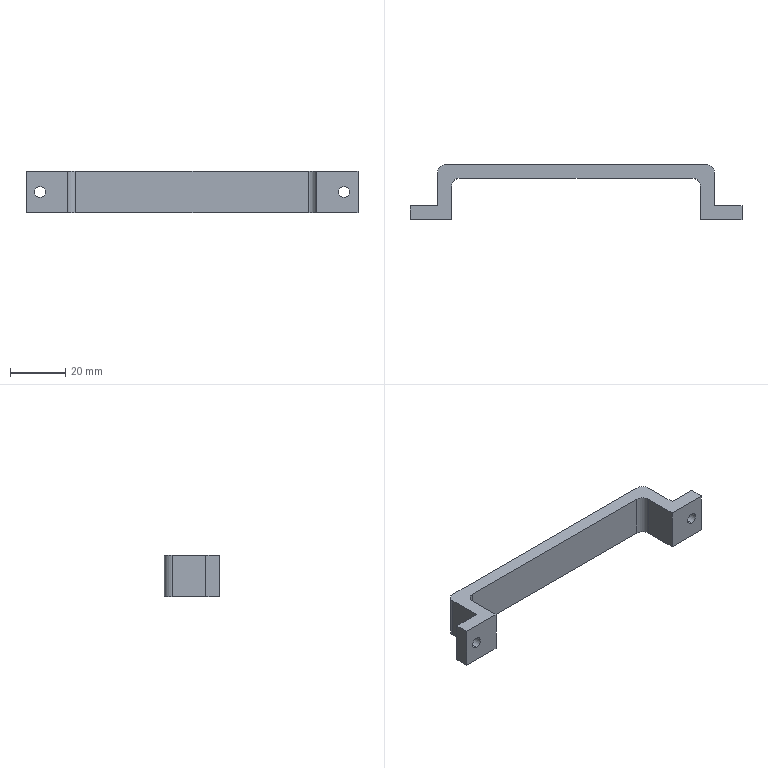Part | SolidWorks | features Extrusion 1, Fillet 1, ICE 1 | 1 solid | 22 faces | box 120 x 20 x 15 mm | volume 11124 mm3 | plane 14 | cylinder 8 | commonest cylinder face diameters 4 x4 6 x4
STEP:
#1=CARTESIAN_POINT('',(115.,0.,5.5));
#2=VERTEX_POINT('',#1);
#3=CARTESIAN_POINT('',(115.,0.,9.5));
#4=VERTEX_POINT('',#3);
#5=CARTESIAN_POINT('',(115.,0.,7.5));
#6=DIRECTION('',(0.,1.,0.));
#7=DIRECTION('',(0.,0.,1.));
#8=AXIS2_PLACEMENT_3D('',#5,#6,#7);
#9=CIRCLE('',#8,2.);
#10=EDGE_CURVE('',#2,#4,#9,.T.);
#11=ORIENTED_EDGE('',*,*,#10,.F.);
#12=CARTESIAN_POINT('',(115.,5.,5.5));
#13=VERTEX_POINT('',#12);
#14=CARTESIAN_POINT('',(115.,-10.,5.5));
#15=DIRECTION('',(0.,1.,0.));
#16=VECTOR('',#15,1000.);
#17=LINE('',#14,#16);
#18=EDGE_CURVE('',#2,#13,#17,.T.);
#19=ORIENTED_EDGE('',*,*,#18,.T.);
#20=CARTESIAN_POINT('',(115.,5.,9.5));
#21=VERTEX_POINT('',#20);
#22=CARTESIAN_POINT('',(115.,5.,7.5));
#23=DIRECTION('',(0.,1.,0.));
#24=DIRECTION('',(0.,0.,1.));
#25=AXIS2_PLACEMENT_3D('',#22,#23,#24);
#26=CIRCLE('',#25,2.);
#27=EDGE_CURVE('',#13,#21,#26,.T.);
#28=ORIENTED_EDGE('',*,*,#27,.T.);
#29=CARTESIAN_POINT('',(115.,-10.,9.5));
#30=DIRECTION('',(0.,1.,0.));
#31=VECTOR('',#30,1000.);
#32=LINE('',#29,#31);
#33=EDGE_CURVE('',#4,#21,#32,.T.);
#34=ORIENTED_EDGE('',*,*,#33,.F.);
#35=EDGE_LOOP('',(#11,#19,#28,#34));
#36=FACE_OUTER_BOUND('',#35,.T.);
#37=CARTESIAN_POINT('',(115.,-10.,7.5));
#38=DIRECTION('',(0.,1.,0.));
#39=DIRECTION('',(0.,0.,1.));
#40=AXIS2_PLACEMENT_3D('',#37,#38,#39);
#41=CYLINDRICAL_SURFACE('',#40,2.);
#42=ADVANCED_FACE('',(#36),#41,.F.);
#43=CARTESIAN_POINT('',(5.,0.,5.5));
#44=VERTEX_POINT('',#43);
#45=CARTESIAN_POINT('',(5.,0.,9.5));
#46=VERTEX_POINT('',#45);
#47=CARTESIAN_POINT('',(5.,0.,7.5));
#48=DIRECTION('',(0.,1.,0.));
#49=DIRECTION('',(0.,0.,1.));
#50=AXIS2_PLACEMENT_3D('',#47,#48,#49);
#51=CIRCLE('',#50,2.);
#52=EDGE_CURVE('',#44,#46,#51,.T.);
#53=ORIENTED_EDGE('',*,*,#52,.F.);
#54=CARTESIAN_POINT('',(5.,5.,5.5));
#55=VERTEX_POINT('',#54);
#56=CARTESIAN_POINT('',(5.,-10.,5.5));
#57=DIRECTION('',(0.,1.,0.));
#58=VECTOR('',#57,1000.);
#59=LINE('',#56,#58);
#60=EDGE_CURVE('',#44,#55,#59,.T.);
#61=ORIENTED_EDGE('',*,*,#60,.T.);
#62=CARTESIAN_POINT('',(5.,5.,9.5));
#63=VERTEX_POINT('',#62);
#64=CARTESIAN_POINT('',(5.,5.,7.5));
#65=DIRECTION('',(0.,1.,0.));
#66=DIRECTION('',(0.,0.,1.));
#67=AXIS2_PLACEMENT_3D('',#64,#65,#66);
#68=CIRCLE('',#67,2.);
#69=EDGE_CURVE('',#55,#63,#68,.T.);
#70=ORIENTED_EDGE('',*,*,#69,.T.);
#71=CARTESIAN_POINT('',(5.,-10.,9.5));
#72=DIRECTION('',(0.,1.,0.));
#73=VECTOR('',#72,1000.);
#74=LINE('',#71,#73);
#75=EDGE_CURVE('',#46,#63,#74,.T.);
#76=ORIENTED_EDGE('',*,*,#75,.F.);
#77=EDGE_LOOP('',(#53,#61,#70,#76));
#78=FACE_OUTER_BOUND('',#77,.T.);
#79=CARTESIAN_POINT('',(5.,-10.,7.5));
#80=DIRECTION('',(0.,1.,0.));
#81=DIRECTION('',(0.,0.,1.));
#82=AXIS2_PLACEMENT_3D('',#79,#80,#81);
#83=CYLINDRICAL_SURFACE('',#82,2.);
#84=ADVANCED_FACE('',(#78),#83,.F.);
#85=CARTESIAN_POINT('',(0.,5.,0.));
#86=VERTEX_POINT('',#85);
#87=CARTESIAN_POINT('',(0.,0.,0.));
#88=VERTEX_POINT('',#87);
#89=CARTESIAN_POINT('',(0.,0.,0.));
#90=DIRECTION('',(0.,-1.,0.));
#91=VECTOR('',#90,1000.);
#92=LINE('',#89,#91);
#93=EDGE_CURVE('',#86,#88,#92,.T.);
#94=ORIENTED_EDGE('',*,*,#93,.T.);
#95=CARTESIAN_POINT('',(0.,0.,15.));
#96=VERTEX_POINT('',#95);
#97=CARTESIAN_POINT('',(0.,0.,15.));
#98=DIRECTION('',(0.,0.,-1.));
#99=VECTOR('',#98,1000.);
#100=LINE('',#97,#99);
#101=EDGE_CURVE('',#96,#88,#100,.T.);
#102=ORIENTED_EDGE('',*,*,#101,.F.);
#103=CARTESIAN_POINT('',(0.,5.,15.));
#104=VERTEX_POINT('',#103);
#105=CARTESIAN_POINT('',(0.,0.,15.));
#106=DIRECTION('',(0.,-1.,0.));
#107=VECTOR('',#106,1000.);
#108=LINE('',#105,#107);
#109=EDGE_CURVE('',#104,#96,#108,.T.);
#110=ORIENTED_EDGE('',*,*,#109,.F.);
#111=CARTESIAN_POINT('',(0.,5.,15.));
#112=DIRECTION('',(0.,0.,-1.));
#113=VECTOR('',#112,1000.);
#114=LINE('',#111,#113);
#115=EDGE_CURVE('',#104,#86,#114,.T.);
#116=ORIENTED_EDGE('',*,*,#115,.T.);
#117=EDGE_LOOP('',(#94,#102,#110,#116));
#118=FACE_OUTER_BOUND('',#117,.T.);
#119=CARTESIAN_POINT('',(0.,0.,15.));
#120=DIRECTION('',(1.,0.,0.));
#121=DIRECTION('',(0.,0.,-1.));
#122=AXIS2_PLACEMENT_3D('',#119,#120,#121);
#123=PLANE('',#122);
#124=ADVANCED_FACE('',(#118),#123,.F.);
#125=CARTESIAN_POINT('',(5.,0.,7.5));
#126=DIRECTION('',(0.,1.,0.));
#127=DIRECTION('',(0.,0.,1.));
#128=AXIS2_PLACEMENT_3D('',#125,#126,#127);
#129=CIRCLE('',#128,2.);
#130=EDGE_CURVE('',#46,#44,#129,.T.);
#131=ORIENTED_EDGE('',*,*,#130,.T.);
#132=ORIENTED_EDGE('',*,*,#52,.T.);
#133=EDGE_LOOP('',(#131,#132));
#134=FACE_BOUND('',#133,.T.);
#135=CARTESIAN_POINT('',(15.,0.,0.));
#136=VERTEX_POINT('',#135);
#137=CARTESIAN_POINT('',(0.,0.,0.));
#138=DIRECTION('',(1.,0.,0.));
#139=VECTOR('',#138,1000.);
#140=LINE('',#137,#139);
#141=EDGE_CURVE('',#88,#136,#140,.T.);
#142=ORIENTED_EDGE('',*,*,#141,.T.);
#143=CARTESIAN_POINT('',(15.,0.,15.));
#144=VERTEX_POINT('',#143);
#145=CARTESIAN_POINT('',(15.,0.,15.));
#146=DIRECTION('',(0.,0.,-1.));
#147=VECTOR('',#146,1000.);
#148=LINE('',#145,#147);
#149=EDGE_CURVE('',#144,#136,#148,.T.);
#150=ORIENTED_EDGE('',*,*,#149,.F.);
#151=CARTESIAN_POINT('',(0.,0.,15.));
#152=DIRECTION('',(1.,0.,0.));
#153=VECTOR('',#152,1000.);
#154=LINE('',#151,#153);
#155=EDGE_CURVE('',#96,#144,#154,.T.);
#156=ORIENTED_EDGE('',*,*,#155,.F.);
#157=ORIENTED_EDGE('',*,*,#101,.T.);
#158=EDGE_LOOP('',(#142,#150,#156,#157));
#159=FACE_OUTER_BOUND('',#158,.T.);
#160=CARTESIAN_POINT('',(0.,0.,15.));
#161=DIRECTION('',(0.,1.,0.));
#162=DIRECTION('',(0.,0.,1.));
#163=AXIS2_PLACEMENT_3D('',#160,#161,#162);
#164=PLANE('',#163);
#165=ADVANCED_FACE('',(#134,#159),#164,.F.);
#166=CARTESIAN_POINT('',(15.,12.,0.));
#167=VERTEX_POINT('',#166);
#168=CARTESIAN_POINT('',(15.,0.,0.));
#169=DIRECTION('',(0.,1.,0.));
#170=VECTOR('',#169,1000.);
#171=LINE('',#168,#170);
#172=EDGE_CURVE('',#136,#167,#171,.T.);
#173=ORIENTED_EDGE('',*,*,#172,.T.);
#174=CARTESIAN_POINT('',(15.,12.,15.));
#175=VERTEX_POINT('',#174);
#176=CARTESIAN_POINT('',(15.,12.,15.));
#177=DIRECTION('',(0.,0.,1.));
#178=VECTOR('',#177,1000.);
#179=LINE('',#176,#178);
#180=EDGE_CURVE('',#167,#175,#179,.T.);
#181=ORIENTED_EDGE('',*,*,#180,.T.);
#182=CARTESIAN_POINT('',(15.,0.,15.));
#183=DIRECTION('',(0.,1.,0.));
#184=VECTOR('',#183,1000.);
#185=LINE('',#182,#184);
#186=EDGE_CURVE('',#144,#175,#185,.T.);
#187=ORIENTED_EDGE('',*,*,#186,.F.);
#188=ORIENTED_EDGE('',*,*,#149,.T.);
#189=EDGE_LOOP('',(#173,#181,#187,#188));
#190=FACE_OUTER_BOUND('',#189,.T.);
#191=CARTESIAN_POINT('',(15.,0.,15.));
#192=DIRECTION('',(-1.,0.,0.));
#193=DIRECTION('',(0.,0.,1.));
#194=AXIS2_PLACEMENT_3D('',#191,#192,#193);
#195=PLANE('',#194);
#196=ADVANCED_FACE('',(#190),#195,.F.);
#197=CARTESIAN_POINT('',(18.,15.,0.));
#198=VERTEX_POINT('',#197);
#199=CARTESIAN_POINT('',(102.,15.,0.));
#200=VERTEX_POINT('',#199);
#201=CARTESIAN_POINT('',(15.,15.,0.));
#202=DIRECTION('',(1.,0.,0.));
#203=VECTOR('',#202,1000.);
#204=LINE('',#201,#203);
#205=EDGE_CURVE('',#198,#200,#204,.T.);
#206=ORIENTED_EDGE('',*,*,#205,.T.);
#207=CARTESIAN_POINT('',(102.,15.,15.));
#208=VERTEX_POINT('',#207);
#209=CARTESIAN_POINT('',(102.,15.,15.));
#210=DIRECTION('',(0.,0.,1.));
#211=VECTOR('',#210,1000.);
#212=LINE('',#209,#211);
#213=EDGE_CURVE('',#200,#208,#212,.T.);
#214=ORIENTED_EDGE('',*,*,#213,.T.);
#215=CARTESIAN_POINT('',(18.,15.,15.));
#216=VERTEX_POINT('',#215);
#217=CARTESIAN_POINT('',(15.,15.,15.));
#218=DIRECTION('',(1.,0.,0.));
#219=VECTOR('',#218,1000.);
#220=LINE('',#217,#219);
#221=EDGE_CURVE('',#216,#208,#220,.T.);
#222=ORIENTED_EDGE('',*,*,#221,.F.);
#223=CARTESIAN_POINT('',(18.,15.,0.));
#224=DIRECTION('',(0.,0.,-1.));
#225=VECTOR('',#224,1000.);
#226=LINE('',#223,#225);
#227=EDGE_CURVE('',#216,#198,#226,.T.);
#228=ORIENTED_EDGE('',*,*,#227,.T.);
#229=EDGE_LOOP('',(#206,#214,#222,#228));
#230=FACE_OUTER_BOUND('',#229,.T.);
#231=CARTESIAN_POINT('',(15.,15.,15.));
#232=DIRECTION('',(0.,1.,0.));
#233=DIRECTION('',(0.,0.,1.));
#234=AXIS2_PLACEMENT_3D('',#231,#232,#233);
#235=PLANE('',#234);
#236=ADVANCED_FACE('',(#230),#235,.F.);
#237=CARTESIAN_POINT('',(105.,12.,15.));
#238=VERTEX_POINT('',#237);
#239=CARTESIAN_POINT('',(105.,0.,15.));
#240=VERTEX_POINT('',#239);
#241=CARTESIAN_POINT('',(105.,15.,15.));
#242=DIRECTION('',(0.,-1.,0.));
#243=VECTOR('',#242,1000.);
#244=LINE('',#241,#243);
#245=EDGE_CURVE('',#238,#240,#244,.T.);
#246=ORIENTED_EDGE('',*,*,#245,.F.);
#247=CARTESIAN_POINT('',(105.,12.,0.));
#248=VERTEX_POINT('',#247);
#249=CARTESIAN_POINT('',(105.,12.,0.));
#250=DIRECTION('',(0.,0.,-1.));
#251=VECTOR('',#250,1000.);
#252=LINE('',#249,#251);
#253=EDGE_CURVE('',#238,#248,#252,.T.);
#254=ORIENTED_EDGE('',*,*,#253,.T.);
#255=CARTESIAN_POINT('',(105.,0.,0.));
#256=VERTEX_POINT('',#255);
#257=CARTESIAN_POINT('',(105.,15.,0.));
#258=DIRECTION('',(0.,-1.,0.));
#259=VECTOR('',#258,1000.);
#260=LINE('',#257,#259);
#261=EDGE_CURVE('',#248,#256,#260,.T.);
#262=ORIENTED_EDGE('',*,*,#261,.T.);
#263=CARTESIAN_POINT('',(105.,0.,15.));
#264=DIRECTION('',(0.,0.,-1.));
#265=VECTOR('',#264,1000.);
#266=LINE('',#263,#265);
#267=EDGE_CURVE('',#240,#256,#266,.T.);
#268=ORIENTED_EDGE('',*,*,#267,.F.);
#269=EDGE_LOOP('',(#246,#254,#262,#268));
#270=FACE_OUTER_BOUND('',#269,.T.);
#271=CARTESIAN_POINT('',(105.,15.,15.));
#272=DIRECTION('',(1.,0.,0.));
#273=DIRECTION('',(0.,0.,-1.));
#274=AXIS2_PLACEMENT_3D('',#271,#272,#273);
#275=PLANE('',#274);
#276=ADVANCED_FACE('',(#270),#275,.F.);
#277=CARTESIAN_POINT('',(115.,0.,7.5));
#278=DIRECTION('',(0.,1.,0.));
#279=DIRECTION('',(0.,0.,1.));
#280=AXIS2_PLACEMENT_3D('',#277,#278,#279);
#281=CIRCLE('',#280,2.);
#282=EDGE_CURVE('',#4,#2,#281,.T.);
#283=ORIENTED_EDGE('',*,*,#282,.T.);
#284=ORIENTED_EDGE('',*,*,#10,.T.);
#285=EDGE_LOOP('',(#283,#284));
#286=FACE_BOUND('',#285,.T.);
#287=CARTESIAN_POINT('',(120.,0.,0.));
#288=VERTEX_POINT('',#287);
#289=CARTESIAN_POINT('',(105.,0.,0.));
#290=DIRECTION('',(1.,0.,0.));
#291=VECTOR('',#290,1000.);
#292=LINE('',#289,#291);
#293=EDGE_CURVE('',#256,#288,#292,.T.);
#294=ORIENTED_EDGE('',*,*,#293,.T.);
#295=CARTESIAN_POINT('',(120.,0.,15.));
#296=VERTEX_POINT('',#295);
#297=CARTESIAN_POINT('',(120.,0.,15.));
#298=DIRECTION('',(0.,0.,-1.));
#299=VECTOR('',#298,1000.);
#300=LINE('',#297,#299);
#301=EDGE_CURVE('',#296,#288,#300,.T.);
#302=ORIENTED_EDGE('',*,*,#301,.F.);
#303=CARTESIAN_POINT('',(105.,0.,15.));
#304=DIRECTION('',(1.,0.,0.));
#305=VECTOR('',#304,1000.);
#306=LINE('',#303,#305);
#307=EDGE_CURVE('',#240,#296,#306,.T.);
#308=ORIENTED_EDGE('',*,*,#307,.F.);
#309=ORIENTED_EDGE('',*,*,#267,.T.);
#310=EDGE_LOOP('',(#294,#302,#308,#309));
#311=FACE_OUTER_BOUND('',#310,.T.);
#312=CARTESIAN_POINT('',(105.,0.,15.));
#313=DIRECTION('',(0.,1.,0.));
#314=DIRECTION('',(0.,0.,1.));
#315=AXIS2_PLACEMENT_3D('',#312,#313,#314);
#316=PLANE('',#315);
#317=ADVANCED_FACE('',(#286,#311),#316,.F.);
#318=CARTESIAN_POINT('',(120.,5.,0.));
#319=VERTEX_POINT('',#318);
#320=CARTESIAN_POINT('',(120.,0.,0.));
#321=DIRECTION('',(0.,1.,0.));
#322=VECTOR('',#321,1000.);
#323=LINE('',#320,#322);
#324=EDGE_CURVE('',#288,#319,#323,.T.);
#325=ORIENTED_EDGE('',*,*,#324,.T.);
#326=CARTESIAN_POINT('',(120.,5.,15.));
#327=VERTEX_POINT('',#326);
#328=CARTESIAN_POINT('',(120.,5.,15.));
#329=DIRECTION('',(0.,0.,-1.));
#330=VECTOR('',#329,1000.);
#331=LINE('',#328,#330);
#332=EDGE_CURVE('',#327,#319,#331,.T.);
#333=ORIENTED_EDGE('',*,*,#332,.F.);
#334=CARTESIAN_POINT('',(120.,0.,15.));
#335=DIRECTION('',(0.,1.,0.));
#336=VECTOR('',#335,1000.);
#337=LINE('',#334,#336);
#338=EDGE_CURVE('',#296,#327,#337,.T.);
#339=ORIENTED_EDGE('',*,*,#338,.F.);
#340=ORIENTED_EDGE('',*,*,#301,.T.);
#341=EDGE_LOOP('',(#325,#333,#339,#340));
#342=FACE_OUTER_BOUND('',#341,.T.);
#343=CARTESIAN_POINT('',(120.,0.,15.));
#344=DIRECTION('',(-1.,0.,0.));
#345=DIRECTION('',(0.,0.,1.));
#346=AXIS2_PLACEMENT_3D('',#343,#344,#345);
#347=PLANE('',#346);
#348=ADVANCED_FACE('',(#342),#347,.F.);
#349=CARTESIAN_POINT('',(115.,5.,7.5));
#350=DIRECTION('',(0.,1.,0.));
#351=DIRECTION('',(0.,0.,1.));
#352=AXIS2_PLACEMENT_3D('',#349,#350,#351);
#353=CIRCLE('',#352,2.);
#354=EDGE_CURVE('',#21,#13,#353,.T.);
#355=ORIENTED_EDGE('',*,*,#354,.F.);
#356=ORIENTED_EDGE('',*,*,#27,.F.);
#357=EDGE_LOOP('',(#355,#356));
#358=FACE_BOUND('',#357,.T.);
#359=CARTESIAN_POINT('',(110.,5.,0.));
#360=VERTEX_POINT('',#359);
#361=CARTESIAN_POINT('',(120.,5.,0.));
#362=DIRECTION('',(-1.,0.,0.));
#363=VECTOR('',#362,1000.);
#364=LINE('',#361,#363);
#365=EDGE_CURVE('',#319,#360,#364,.T.);
#366=ORIENTED_EDGE('',*,*,#365,.T.);
#367=CARTESIAN_POINT('',(110.,5.,15.));
#368=VERTEX_POINT('',#367);
#369=CARTESIAN_POINT('',(110.,5.,15.));
#370=DIRECTION('',(0.,0.,-1.));
#371=VECTOR('',#370,1000.);
#372=LINE('',#369,#371);
#373=EDGE_CURVE('',#368,#360,#372,.T.);
#374=ORIENTED_EDGE('',*,*,#373,.F.);
#375=CARTESIAN_POINT('',(120.,5.,15.));
#376=DIRECTION('',(-1.,0.,0.));
#377=VECTOR('',#376,1000.);
#378=LINE('',#375,#377);
#379=EDGE_CURVE('',#327,#368,#378,.T.);
#380=ORIENTED_EDGE('',*,*,#379,.F.);
#381=ORIENTED_EDGE('',*,*,#332,.T.);
#382=EDGE_LOOP('',(#366,#374,#380,#381));
#383=FACE_OUTER_BOUND('',#382,.T.);
#384=CARTESIAN_POINT('',(120.,5.,15.));
#385=DIRECTION('',(0.,-1.,0.));
#386=DIRECTION('',(1.,0.,0.));
#387=AXIS2_PLACEMENT_3D('',#384,#385,#386);
#388=PLANE('',#387);
#389=ADVANCED_FACE('',(#358,#383),#388,.F.);
#390=CARTESIAN_POINT('',(110.,17.,0.));
#391=VERTEX_POINT('',#390);
#392=CARTESIAN_POINT('',(110.,5.,0.));
#393=DIRECTION('',(0.,1.,0.));
#394=VECTOR('',#393,1000.);
#395=LINE('',#392,#394);
#396=EDGE_CURVE('',#360,#391,#395,.T.);
#397=ORIENTED_EDGE('',*,*,#396,.T.);
#398=CARTESIAN_POINT('',(110.,17.,15.));
#399=VERTEX_POINT('',#398);
#400=CARTESIAN_POINT('',(110.,17.,15.));
#401=DIRECTION('',(0.,0.,1.));
#402=VECTOR('',#401,1000.);
#403=LINE('',#400,#402);
#404=EDGE_CURVE('',#391,#399,#403,.T.);
#405=ORIENTED_EDGE('',*,*,#404,.T.);
#406=CARTESIAN_POINT('',(110.,5.,15.));
#407=DIRECTION('',(0.,1.,0.));
#408=VECTOR('',#407,1000.);
#409=LINE('',#406,#408);
#410=EDGE_CURVE('',#368,#399,#409,.T.);
#411=ORIENTED_EDGE('',*,*,#410,.F.);
#412=ORIENTED_EDGE('',*,*,#373,.T.);
#413=EDGE_LOOP('',(#397,#405,#411,#412));
#414=FACE_OUTER_BOUND('',#413,.T.);
#415=CARTESIAN_POINT('',(110.,5.,15.));
#416=DIRECTION('',(-1.,0.,0.));
#417=DIRECTION('',(0.,0.,1.));
#418=AXIS2_PLACEMENT_3D('',#415,#416,#417);
#419=PLANE('',#418);
#420=ADVANCED_FACE('',(#414),#419,.F.);
#421=CARTESIAN_POINT('',(107.,20.,15.));
#422=VERTEX_POINT('',#421);
#423=CARTESIAN_POINT('',(13.,20.,15.));
#424=VERTEX_POINT('',#423);
#425=CARTESIAN_POINT('',(10.,20.,15.));
#426=DIRECTION('',(-1.,0.,0.));
#427=VECTOR('',#426,1000.);
#428=LINE('',#425,#427);
#429=EDGE_CURVE('',#422,#424,#428,.T.);
#430=ORIENTED_EDGE('',*,*,#429,.F.);
#431=CARTESIAN_POINT('',(107.,20.,0.));
#432=VERTEX_POINT('',#431);
#433=CARTESIAN_POINT('',(107.,20.,15.));
#434=DIRECTION('',(0.,0.,-1.));
#435=VECTOR('',#434,1000.);
#436=LINE('',#433,#435);
#437=EDGE_CURVE('',#422,#432,#436,.T.);
#438=ORIENTED_EDGE('',*,*,#437,.T.);
#439=CARTESIAN_POINT('',(13.,20.,0.));
#440=VERTEX_POINT('',#439);
#441=CARTESIAN_POINT('',(10.,20.,0.));
#442=DIRECTION('',(-1.,0.,0.));
#443=VECTOR('',#442,1000.);
#444=LINE('',#441,#443);
#445=EDGE_CURVE('',#432,#440,#444,.T.);
#446=ORIENTED_EDGE('',*,*,#445,.T.);
#447=CARTESIAN_POINT('',(13.,20.,15.));
#448=DIRECTION('',(0.,0.,1.));
#449=VECTOR('',#448,1000.);
#450=LINE('',#447,#449);
#451=EDGE_CURVE('',#440,#424,#450,.T.);
#452=ORIENTED_EDGE('',*,*,#451,.T.);
#453=EDGE_LOOP('',(#430,#438,#446,#452));
#454=FACE_OUTER_BOUND('',#453,.T.);
#455=CARTESIAN_POINT('',(10.,20.,15.));
#456=DIRECTION('',(0.,-1.,0.));
#457=DIRECTION('',(0.,0.,-1.));
#458=AXIS2_PLACEMENT_3D('',#455,#456,#457);
#459=PLANE('',#458);
#460=ADVANCED_FACE('',(#454),#459,.F.);
#461=CARTESIAN_POINT('',(10.,17.,15.));
#462=VERTEX_POINT('',#461);
#463=CARTESIAN_POINT('',(10.,5.,15.));
#464=VERTEX_POINT('',#463);
#465=CARTESIAN_POINT('',(10.,5.,15.));
#466=DIRECTION('',(0.,-1.,0.));
#467=VECTOR('',#466,1000.);
#468=LINE('',#465,#467);
#469=EDGE_CURVE('',#462,#464,#468,.T.);
#470=ORIENTED_EDGE('',*,*,#469,.F.);
#471=CARTESIAN_POINT('',(10.,17.,0.));
#472=VERTEX_POINT('',#471);
#473=CARTESIAN_POINT('',(10.,17.,15.));
#474=DIRECTION('',(0.,0.,-1.));
#475=VECTOR('',#474,1000.);
#476=LINE('',#473,#475);
#477=EDGE_CURVE('',#462,#472,#476,.T.);
#478=ORIENTED_EDGE('',*,*,#477,.T.);
#479=CARTESIAN_POINT('',(10.,5.,0.));
#480=VERTEX_POINT('',#479);
#481=CARTESIAN_POINT('',(10.,5.,0.));
#482=DIRECTION('',(0.,-1.,0.));
#483=VECTOR('',#482,1000.);
#484=LINE('',#481,#483);
#485=EDGE_CURVE('',#472,#480,#484,.T.);
#486=ORIENTED_EDGE('',*,*,#485,.T.);
#487=CARTESIAN_POINT('',(10.,5.,15.));
#488=DIRECTION('',(0.,0.,-1.));
#489=VECTOR('',#488,1000.);
#490=LINE('',#487,#489);
#491=EDGE_CURVE('',#464,#480,#490,.T.);
#492=ORIENTED_EDGE('',*,*,#491,.F.);
#493=EDGE_LOOP('',(#470,#478,#486,#492));
#494=FACE_OUTER_BOUND('',#493,.T.);
#495=CARTESIAN_POINT('',(10.,5.,15.));
#496=DIRECTION('',(1.,0.,0.));
#497=DIRECTION('',(0.,0.,-1.));
#498=AXIS2_PLACEMENT_3D('',#495,#496,#497);
#499=PLANE('',#498);
#500=ADVANCED_FACE('',(#494),#499,.F.);
#501=CARTESIAN_POINT('',(5.,5.,7.5));
#502=DIRECTION('',(0.,1.,0.));
#503=DIRECTION('',(0.,0.,1.));
#504=AXIS2_PLACEMENT_3D('',#501,#502,#503);
#505=CIRCLE('',#504,2.);
#506=EDGE_CURVE('',#63,#55,#505,.T.);
#507=ORIENTED_EDGE('',*,*,#506,.F.);
#508=ORIENTED_EDGE('',*,*,#69,.F.);
#509=EDGE_LOOP('',(#507,#508));
#510=FACE_BOUND('',#509,.T.);
#511=CARTESIAN_POINT('',(0.,5.,0.));
#512=DIRECTION('',(-1.,0.,0.));
#513=VECTOR('',#512,1000.);
#514=LINE('',#511,#513);
#515=EDGE_CURVE('',#480,#86,#514,.T.);
#516=ORIENTED_EDGE('',*,*,#515,.T.);
#517=ORIENTED_EDGE('',*,*,#115,.F.);
#518=CARTESIAN_POINT('',(0.,5.,15.));
#519=DIRECTION('',(-1.,0.,0.));
#520=VECTOR('',#519,1000.);
#521=LINE('',#518,#520);
#522=EDGE_CURVE('',#464,#104,#521,.T.);
#523=ORIENTED_EDGE('',*,*,#522,.F.);
#524=ORIENTED_EDGE('',*,*,#491,.T.);
#525=EDGE_LOOP('',(#516,#517,#523,#524));
#526=FACE_OUTER_BOUND('',#525,.T.);
#527=CARTESIAN_POINT('',(0.,5.,15.));
#528=DIRECTION('',(0.,-1.,0.));
#529=DIRECTION('',(0.,0.,-1.));
#530=AXIS2_PLACEMENT_3D('',#527,#528,#529);
#531=PLANE('',#530);
#532=ADVANCED_FACE('',(#510,#526),#531,.F.);
#533=ORIENTED_EDGE('',*,*,#410,.T.);
#534=CARTESIAN_POINT('',(107.,17.,15.));
#535=DIRECTION('',(0.,0.,1.));
#536=DIRECTION('',(-1.,0.,0.));
#537=AXIS2_PLACEMENT_3D('',#534,#535,#536);
#538=CIRCLE('',#537,3.);
#539=EDGE_CURVE('',#399,#422,#538,.T.);
#540=ORIENTED_EDGE('',*,*,#539,.T.);
#541=ORIENTED_EDGE('',*,*,#429,.T.);
#542=CARTESIAN_POINT('',(13.,17.,15.));
#543=DIRECTION('',(0.,0.,1.));
#544=DIRECTION('',(-1.,0.,0.));
#545=AXIS2_PLACEMENT_3D('',#542,#543,#544);
#546=CIRCLE('',#545,3.);
#547=EDGE_CURVE('',#424,#462,#546,.T.);
#548=ORIENTED_EDGE('',*,*,#547,.T.);
#549=ORIENTED_EDGE('',*,*,#469,.T.);
#550=ORIENTED_EDGE('',*,*,#522,.T.);
#551=ORIENTED_EDGE('',*,*,#109,.T.);
#552=ORIENTED_EDGE('',*,*,#155,.T.);
#553=ORIENTED_EDGE('',*,*,#186,.T.);
#554=CARTESIAN_POINT('',(18.,12.,15.));
#555=DIRECTION('',(0.,0.,-1.));
#556=DIRECTION('',(-1.,0.,0.));
#557=AXIS2_PLACEMENT_3D('',#554,#555,#556);
#558=CIRCLE('',#557,3.);
#559=EDGE_CURVE('',#175,#216,#558,.T.);
#560=ORIENTED_EDGE('',*,*,#559,.T.);
#561=ORIENTED_EDGE('',*,*,#221,.T.);
#562=CARTESIAN_POINT('',(102.,12.,15.));
#563=DIRECTION('',(0.,0.,-1.));
#564=DIRECTION('',(-1.,0.,0.));
#565=AXIS2_PLACEMENT_3D('',#562,#563,#564);
#566=CIRCLE('',#565,3.);
#567=EDGE_CURVE('',#208,#238,#566,.T.);
#568=ORIENTED_EDGE('',*,*,#567,.T.);
#569=ORIENTED_EDGE('',*,*,#245,.T.);
#570=ORIENTED_EDGE('',*,*,#307,.T.);
#571=ORIENTED_EDGE('',*,*,#338,.T.);
#572=ORIENTED_EDGE('',*,*,#379,.T.);
#573=EDGE_LOOP('',(#533,#540,#541,#548,#549,#550,#551,#552,#553,#560,#561,#568,#569,#570,#571,#572));
#574=FACE_OUTER_BOUND('',#573,.T.);
#575=CARTESIAN_POINT('',(0.,5.,15.));
#576=DIRECTION('',(0.,0.,-1.));
#577=DIRECTION('',(-1.,0.,0.));
#578=AXIS2_PLACEMENT_3D('',#575,#576,#577);
#579=PLANE('',#578);
#580=ADVANCED_FACE('',(#574),#579,.F.);
#581=ORIENTED_EDGE('',*,*,#445,.F.);
#582=CARTESIAN_POINT('',(107.,17.,0.));
#583=DIRECTION('',(0.,0.,-1.));
#584=DIRECTION('',(-1.,0.,0.));
#585=AXIS2_PLACEMENT_3D('',#582,#583,#584);
#586=CIRCLE('',#585,3.);
#587=EDGE_CURVE('',#432,#391,#586,.T.);
#588=ORIENTED_EDGE('',*,*,#587,.T.);
#589=ORIENTED_EDGE('',*,*,#396,.F.);
#590=ORIENTED_EDGE('',*,*,#365,.F.);
#591=ORIENTED_EDGE('',*,*,#324,.F.);
#592=ORIENTED_EDGE('',*,*,#293,.F.);
#593=ORIENTED_EDGE('',*,*,#261,.F.);
#594=CARTESIAN_POINT('',(102.,12.,0.));
#595=DIRECTION('',(0.,0.,1.));
#596=DIRECTION('',(-1.,0.,0.));
#597=AXIS2_PLACEMENT_3D('',#594,#595,#596);
#598=CIRCLE('',#597,3.);
#599=EDGE_CURVE('',#248,#200,#598,.T.);
#600=ORIENTED_EDGE('',*,*,#599,.T.);
#601=ORIENTED_EDGE('',*,*,#205,.F.);
#602=CARTESIAN_POINT('',(18.,12.,0.));
#603=DIRECTION('',(0.,0.,1.));
#604=DIRECTION('',(-1.,0.,0.));
#605=AXIS2_PLACEMENT_3D('',#602,#603,#604);
#606=CIRCLE('',#605,3.);
#607=EDGE_CURVE('',#198,#167,#606,.T.);
#608=ORIENTED_EDGE('',*,*,#607,.T.);
#609=ORIENTED_EDGE('',*,*,#172,.F.);
#610=ORIENTED_EDGE('',*,*,#141,.F.);
#611=ORIENTED_EDGE('',*,*,#93,.F.);
#612=ORIENTED_EDGE('',*,*,#515,.F.);
#613=ORIENTED_EDGE('',*,*,#485,.F.);
#614=CARTESIAN_POINT('',(13.,17.,0.));
#615=DIRECTION('',(0.,0.,-1.));
#616=DIRECTION('',(-1.,0.,0.));
#617=AXIS2_PLACEMENT_3D('',#614,#615,#616);
#618=CIRCLE('',#617,3.);
#619=EDGE_CURVE('',#472,#440,#618,.T.);
#620=ORIENTED_EDGE('',*,*,#619,.T.);
#621=EDGE_LOOP('',(#581,#588,#589,#590,#591,#592,#593,#600,#601,#608,#609,#610,#611,#612,#613,#620));
#622=FACE_OUTER_BOUND('',#621,.T.);
#623=CARTESIAN_POINT('',(0.,5.,0.));
#624=DIRECTION('',(0.,0.,-1.));
#625=DIRECTION('',(-1.,0.,0.));
#626=AXIS2_PLACEMENT_3D('',#623,#624,#625);
#627=PLANE('',#626);
#628=ADVANCED_FACE('',(#622),#627,.T.);
#629=ORIENTED_EDGE('',*,*,#60,.F.);
#630=ORIENTED_EDGE('',*,*,#130,.F.);
#631=ORIENTED_EDGE('',*,*,#75,.T.);
#632=ORIENTED_EDGE('',*,*,#506,.T.);
#633=EDGE_LOOP('',(#629,#630,#631,#632));
#634=FACE_OUTER_BOUND('',#633,.T.);
#635=CARTESIAN_POINT('',(5.,-10.,7.5));
#636=DIRECTION('',(0.,1.,0.));
#637=DIRECTION('',(0.,0.,1.));
#638=AXIS2_PLACEMENT_3D('',#635,#636,#637);
#639=CYLINDRICAL_SURFACE('',#638,2.);
#640=ADVANCED_FACE('',(#634),#639,.F.);
#641=ORIENTED_EDGE('',*,*,#18,.F.);
#642=ORIENTED_EDGE('',*,*,#282,.F.);
#643=ORIENTED_EDGE('',*,*,#33,.T.);
#644=ORIENTED_EDGE('',*,*,#354,.T.);
#645=EDGE_LOOP('',(#641,#642,#643,#644));
#646=FACE_OUTER_BOUND('',#645,.T.);
#647=CARTESIAN_POINT('',(115.,-10.,7.5));
#648=DIRECTION('',(0.,1.,0.));
#649=DIRECTION('',(0.,0.,1.));
#650=AXIS2_PLACEMENT_3D('',#647,#648,#649);
#651=CYLINDRICAL_SURFACE('',#650,2.);
#652=ADVANCED_FACE('',(#646),#651,.F.);
#653=ORIENTED_EDGE('',*,*,#567,.F.);
#654=ORIENTED_EDGE('',*,*,#213,.F.);
#655=ORIENTED_EDGE('',*,*,#599,.F.);
#656=ORIENTED_EDGE('',*,*,#253,.F.);
#657=EDGE_LOOP('',(#653,#654,#655,#656));
#658=FACE_OUTER_BOUND('',#657,.T.);
#659=CARTESIAN_POINT('',(102.,12.,15.));
#660=DIRECTION('',(0.,0.,1.));
#661=DIRECTION('',(1.,0.,0.));
#662=AXIS2_PLACEMENT_3D('',#659,#660,#661);
#663=CYLINDRICAL_SURFACE('',#662,3.);
#664=ADVANCED_FACE('',(#658),#663,.F.);
#665=ORIENTED_EDGE('',*,*,#559,.F.);
#666=ORIENTED_EDGE('',*,*,#180,.F.);
#667=ORIENTED_EDGE('',*,*,#607,.F.);
#668=ORIENTED_EDGE('',*,*,#227,.F.);
#669=EDGE_LOOP('',(#665,#666,#667,#668));
#670=FACE_OUTER_BOUND('',#669,.T.);
#671=CARTESIAN_POINT('',(18.,12.,15.));
#672=DIRECTION('',(0.,0.,1.));
#673=DIRECTION('',(1.,0.,0.));
#674=AXIS2_PLACEMENT_3D('',#671,#672,#673);
#675=CYLINDRICAL_SURFACE('',#674,3.);
#676=ADVANCED_FACE('',(#670),#675,.F.);
#677=ORIENTED_EDGE('',*,*,#539,.F.);
#678=ORIENTED_EDGE('',*,*,#404,.F.);
#679=ORIENTED_EDGE('',*,*,#587,.F.);
#680=ORIENTED_EDGE('',*,*,#437,.F.);
#681=EDGE_LOOP('',(#677,#678,#679,#680));
#682=FACE_OUTER_BOUND('',#681,.T.);
#683=CARTESIAN_POINT('',(107.,17.,15.));
#684=DIRECTION('',(0.,0.,-1.));
#685=DIRECTION('',(-1.,0.,0.));
#686=AXIS2_PLACEMENT_3D('',#683,#684,#685);
#687=CYLINDRICAL_SURFACE('',#686,3.);
#688=ADVANCED_FACE('',(#682),#687,.T.);
#689=ORIENTED_EDGE('',*,*,#547,.F.);
#690=ORIENTED_EDGE('',*,*,#451,.F.);
#691=ORIENTED_EDGE('',*,*,#619,.F.);
#692=ORIENTED_EDGE('',*,*,#477,.F.);
#693=EDGE_LOOP('',(#689,#690,#691,#692));
#694=FACE_OUTER_BOUND('',#693,.T.);
#695=CARTESIAN_POINT('',(13.,17.,15.));
#696=DIRECTION('',(0.,0.,-1.));
#697=DIRECTION('',(-1.,0.,0.));
#698=AXIS2_PLACEMENT_3D('',#695,#696,#697);
#699=CYLINDRICAL_SURFACE('',#698,3.);
#700=ADVANCED_FACE('',(#694),#699,.T.);
#701=CLOSED_SHELL('',(#42,#84,#124,#165,#196,#236,#276,#317,#348,#389,#420,#460,#500,#532,#580,#628,#640,#652,#664,#676,#688,#700));
#702=MANIFOLD_SOLID_BREP('',#701);
#703=CARTESIAN_POINT('',(0.,0.,0.));
#704=DIRECTION('',(0.,0.,1.));
#705=DIRECTION('',(1.,0.,0.));
#706=AXIS2_PLACEMENT_3D('',#703,#704,#705);
#707=(LENGTH_UNIT()NAMED_UNIT(*)SI_UNIT(.MILLI.,.METRE.));
#708=UNCERTAINTY_MEASURE_WITH_UNIT(LENGTH_MEASURE(0.00001),#707,'','');
#709=(NAMED_UNIT(*)PLANE_ANGLE_UNIT()SI_UNIT($,.RADIAN.));
#710=(NAMED_UNIT(*)SI_UNIT($,.STERADIAN.)SOLID_ANGLE_UNIT());
#711=(GEOMETRIC_REPRESENTATION_CONTEXT(3)GLOBAL_UNCERTAINTY_ASSIGNED_CONTEXT((#708))GLOBAL_UNIT_ASSIGNED_CONTEXT((#707,#709,#710))REPRESENTATION_CONTEXT('',''));
#712=ADVANCED_BREP_SHAPE_REPRESENTATION('',(#702,#706),#711);